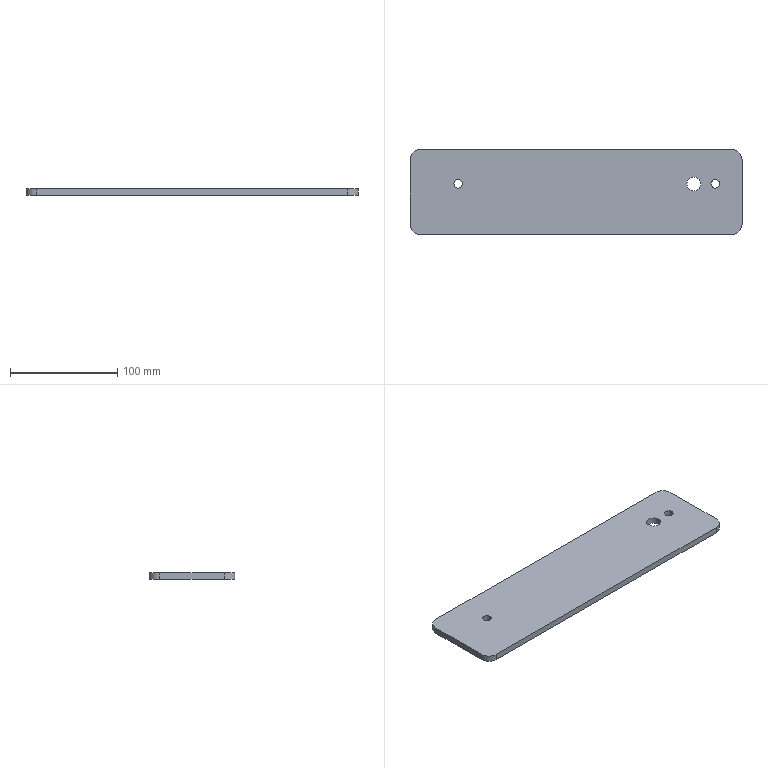Part | SolidWorks | features FlatPattern 1, SMBaseFlange 1, SheetMetal 1 | 1 solid | 16 faces | box 310 x 80 x 6 mm | volume 146885 mm3 | cylinder 10 | plane 6 | commonest cylinder face diameters 8 x4 20 x4 13 x2
STEP:
#1=CARTESIAN_POINT('',(-1216.5,-927.5,6.));
#2=VERTEX_POINT('',#1);
#3=CARTESIAN_POINT('',(-1203.5,-927.5,6.));
#4=VERTEX_POINT('',#3);
#5=CARTESIAN_POINT('',(-1210.,-927.5,6.));
#6=DIRECTION('',(0.,0.,1.));
#7=DIRECTION('',(1.,0.,0.));
#8=AXIS2_PLACEMENT_3D('',#5,#6,#7);
#9=CIRCLE('',#8,6.5);
#10=EDGE_CURVE('',#2,#4,#9,.T.);
#11=ORIENTED_EDGE('',*,*,#10,.T.);
#12=CARTESIAN_POINT('',(-1203.5,-927.5,0.));
#13=VERTEX_POINT('',#12);
#14=CARTESIAN_POINT('',(-1203.5,-927.5,6.));
#15=DIRECTION('',(0.,0.,-1.));
#16=VECTOR('',#15,1000.);
#17=LINE('',#14,#16);
#18=EDGE_CURVE('',#4,#13,#17,.T.);
#19=ORIENTED_EDGE('',*,*,#18,.T.);
#20=CARTESIAN_POINT('',(-1216.5,-927.5,0.));
#21=VERTEX_POINT('',#20);
#22=CARTESIAN_POINT('',(-1210.,-927.5,0.));
#23=DIRECTION('',(0.,0.,1.));
#24=DIRECTION('',(1.,0.,0.));
#25=AXIS2_PLACEMENT_3D('',#22,#23,#24);
#26=CIRCLE('',#25,6.5);
#27=EDGE_CURVE('',#21,#13,#26,.T.);
#28=ORIENTED_EDGE('',*,*,#27,.F.);
#29=CARTESIAN_POINT('',(-1216.5,-927.5,6.));
#30=DIRECTION('',(0.,0.,-1.));
#31=VECTOR('',#30,1000.);
#32=LINE('',#29,#31);
#33=EDGE_CURVE('',#2,#21,#32,.T.);
#34=ORIENTED_EDGE('',*,*,#33,.F.);
#35=EDGE_LOOP('',(#11,#19,#28,#34));
#36=FACE_OUTER_BOUND('',#35,.T.);
#37=CARTESIAN_POINT('',(-1210.,-927.5,6.));
#38=DIRECTION('',(0.,0.,-1.));
#39=DIRECTION('',(-1.,0.,0.));
#40=AXIS2_PLACEMENT_3D('',#37,#38,#39);
#41=CYLINDRICAL_SURFACE('',#40,6.5);
#42=ADVANCED_FACE('',(#36),#41,.F.);
#43=CARTESIAN_POINT('',(-1194.,-927.5,6.));
#44=VERTEX_POINT('',#43);
#45=CARTESIAN_POINT('',(-1186.,-927.5,6.));
#46=VERTEX_POINT('',#45);
#47=CARTESIAN_POINT('',(-1190.,-927.5,6.));
#48=DIRECTION('',(0.,0.,1.));
#49=DIRECTION('',(1.,0.,0.));
#50=AXIS2_PLACEMENT_3D('',#47,#48,#49);
#51=CIRCLE('',#50,4.);
#52=EDGE_CURVE('',#44,#46,#51,.T.);
#53=ORIENTED_EDGE('',*,*,#52,.T.);
#54=CARTESIAN_POINT('',(-1186.,-927.5,0.));
#55=VERTEX_POINT('',#54);
#56=CARTESIAN_POINT('',(-1186.,-927.5,6.));
#57=DIRECTION('',(0.,0.,-1.));
#58=VECTOR('',#57,1000.);
#59=LINE('',#56,#58);
#60=EDGE_CURVE('',#46,#55,#59,.T.);
#61=ORIENTED_EDGE('',*,*,#60,.T.);
#62=CARTESIAN_POINT('',(-1194.,-927.5,0.));
#63=VERTEX_POINT('',#62);
#64=CARTESIAN_POINT('',(-1190.,-927.5,0.));
#65=DIRECTION('',(0.,0.,1.));
#66=DIRECTION('',(1.,0.,0.));
#67=AXIS2_PLACEMENT_3D('',#64,#65,#66);
#68=CIRCLE('',#67,4.);
#69=EDGE_CURVE('',#63,#55,#68,.T.);
#70=ORIENTED_EDGE('',*,*,#69,.F.);
#71=CARTESIAN_POINT('',(-1194.,-927.5,6.));
#72=DIRECTION('',(0.,0.,-1.));
#73=VECTOR('',#72,1000.);
#74=LINE('',#71,#73);
#75=EDGE_CURVE('',#44,#63,#74,.T.);
#76=ORIENTED_EDGE('',*,*,#75,.F.);
#77=EDGE_LOOP('',(#53,#61,#70,#76));
#78=FACE_OUTER_BOUND('',#77,.T.);
#79=CARTESIAN_POINT('',(-1190.,-927.5,6.));
#80=DIRECTION('',(0.,0.,-1.));
#81=DIRECTION('',(-1.,0.,0.));
#82=AXIS2_PLACEMENT_3D('',#79,#80,#81);
#83=CYLINDRICAL_SURFACE('',#82,4.);
#84=ADVANCED_FACE('',(#78),#83,.F.);
#85=CARTESIAN_POINT('',(-1434.,-927.5,6.));
#86=VERTEX_POINT('',#85);
#87=CARTESIAN_POINT('',(-1426.,-927.5,6.));
#88=VERTEX_POINT('',#87);
#89=CARTESIAN_POINT('',(-1430.,-927.5,6.));
#90=DIRECTION('',(0.,0.,1.));
#91=DIRECTION('',(1.,0.,0.));
#92=AXIS2_PLACEMENT_3D('',#89,#90,#91);
#93=CIRCLE('',#92,4.);
#94=EDGE_CURVE('',#86,#88,#93,.T.);
#95=ORIENTED_EDGE('',*,*,#94,.T.);
#96=CARTESIAN_POINT('',(-1426.,-927.5,0.));
#97=VERTEX_POINT('',#96);
#98=CARTESIAN_POINT('',(-1426.,-927.5,6.));
#99=DIRECTION('',(0.,0.,-1.));
#100=VECTOR('',#99,1000.);
#101=LINE('',#98,#100);
#102=EDGE_CURVE('',#88,#97,#101,.T.);
#103=ORIENTED_EDGE('',*,*,#102,.T.);
#104=CARTESIAN_POINT('',(-1434.,-927.5,0.));
#105=VERTEX_POINT('',#104);
#106=CARTESIAN_POINT('',(-1430.,-927.5,0.));
#107=DIRECTION('',(0.,0.,1.));
#108=DIRECTION('',(1.,0.,0.));
#109=AXIS2_PLACEMENT_3D('',#106,#107,#108);
#110=CIRCLE('',#109,4.);
#111=EDGE_CURVE('',#105,#97,#110,.T.);
#112=ORIENTED_EDGE('',*,*,#111,.F.);
#113=CARTESIAN_POINT('',(-1434.,-927.5,6.));
#114=DIRECTION('',(0.,0.,-1.));
#115=VECTOR('',#114,1000.);
#116=LINE('',#113,#115);
#117=EDGE_CURVE('',#86,#105,#116,.T.);
#118=ORIENTED_EDGE('',*,*,#117,.F.);
#119=EDGE_LOOP('',(#95,#103,#112,#118));
#120=FACE_OUTER_BOUND('',#119,.T.);
#121=CARTESIAN_POINT('',(-1430.,-927.5,6.));
#122=DIRECTION('',(0.,0.,-1.));
#123=DIRECTION('',(-1.,0.,0.));
#124=AXIS2_PLACEMENT_3D('',#121,#122,#123);
#125=CYLINDRICAL_SURFACE('',#124,4.);
#126=ADVANCED_FACE('',(#120),#125,.F.);
#127=CARTESIAN_POINT('',(-1165.,-905.,6.));
#128=VERTEX_POINT('',#127);
#129=CARTESIAN_POINT('',(-1175.,-895.,6.));
#130=VERTEX_POINT('',#129);
#131=CARTESIAN_POINT('',(-1175.,-905.,6.));
#132=DIRECTION('',(0.,0.,1.));
#133=DIRECTION('',(-1.,0.,0.));
#134=AXIS2_PLACEMENT_3D('',#131,#132,#133);
#135=CIRCLE('',#134,10.);
#136=EDGE_CURVE('',#128,#130,#135,.T.);
#137=ORIENTED_EDGE('',*,*,#136,.T.);
#138=CARTESIAN_POINT('',(-1465.,-895.,6.));
#139=VERTEX_POINT('',#138);
#140=CARTESIAN_POINT('',(-1465.,-895.,6.));
#141=DIRECTION('',(-1.,0.,0.));
#142=VECTOR('',#141,1000.);
#143=LINE('',#140,#142);
#144=EDGE_CURVE('',#130,#139,#143,.T.);
#145=ORIENTED_EDGE('',*,*,#144,.T.);
#146=CARTESIAN_POINT('',(-1475.,-905.,6.));
#147=VERTEX_POINT('',#146);
#148=CARTESIAN_POINT('',(-1465.,-905.,6.));
#149=DIRECTION('',(0.,0.,1.));
#150=DIRECTION('',(-1.,0.,0.));
#151=AXIS2_PLACEMENT_3D('',#148,#149,#150);
#152=CIRCLE('',#151,10.);
#153=EDGE_CURVE('',#139,#147,#152,.T.);
#154=ORIENTED_EDGE('',*,*,#153,.T.);
#155=CARTESIAN_POINT('',(-1475.,-965.,6.));
#156=VERTEX_POINT('',#155);
#157=CARTESIAN_POINT('',(-1475.,-965.,6.));
#158=DIRECTION('',(0.,-1.,0.));
#159=VECTOR('',#158,1000.);
#160=LINE('',#157,#159);
#161=EDGE_CURVE('',#147,#156,#160,.T.);
#162=ORIENTED_EDGE('',*,*,#161,.T.);
#163=CARTESIAN_POINT('',(-1465.,-975.,6.));
#164=VERTEX_POINT('',#163);
#165=CARTESIAN_POINT('',(-1465.,-965.,6.));
#166=DIRECTION('',(0.,0.,1.));
#167=DIRECTION('',(-1.,0.,0.));
#168=AXIS2_PLACEMENT_3D('',#165,#166,#167);
#169=CIRCLE('',#168,10.);
#170=EDGE_CURVE('',#156,#164,#169,.T.);
#171=ORIENTED_EDGE('',*,*,#170,.T.);
#172=CARTESIAN_POINT('',(-1175.,-975.,6.));
#173=VERTEX_POINT('',#172);
#174=CARTESIAN_POINT('',(-1465.,-975.,6.));
#175=DIRECTION('',(1.,0.,0.));
#176=VECTOR('',#175,1000.);
#177=LINE('',#174,#176);
#178=EDGE_CURVE('',#164,#173,#177,.T.);
#179=ORIENTED_EDGE('',*,*,#178,.T.);
#180=CARTESIAN_POINT('',(-1165.,-965.,6.));
#181=VERTEX_POINT('',#180);
#182=CARTESIAN_POINT('',(-1175.,-965.,6.));
#183=DIRECTION('',(0.,0.,1.));
#184=DIRECTION('',(1.,0.,0.));
#185=AXIS2_PLACEMENT_3D('',#182,#183,#184);
#186=CIRCLE('',#185,10.);
#187=EDGE_CURVE('',#173,#181,#186,.T.);
#188=ORIENTED_EDGE('',*,*,#187,.T.);
#189=CARTESIAN_POINT('',(-1165.,-965.,6.));
#190=DIRECTION('',(0.,1.,0.));
#191=VECTOR('',#190,1000.);
#192=LINE('',#189,#191);
#193=EDGE_CURVE('',#181,#128,#192,.T.);
#194=ORIENTED_EDGE('',*,*,#193,.T.);
#195=EDGE_LOOP('',(#137,#145,#154,#162,#171,#179,#188,#194));
#196=FACE_OUTER_BOUND('',#195,.T.);
#197=ORIENTED_EDGE('',*,*,#94,.F.);
#198=CARTESIAN_POINT('',(-1430.,-927.5,6.));
#199=DIRECTION('',(0.,0.,1.));
#200=DIRECTION('',(1.,0.,0.));
#201=AXIS2_PLACEMENT_3D('',#198,#199,#200);
#202=CIRCLE('',#201,4.);
#203=EDGE_CURVE('',#88,#86,#202,.T.);
#204=ORIENTED_EDGE('',*,*,#203,.F.);
#205=EDGE_LOOP('',(#197,#204));
#206=FACE_BOUND('',#205,.T.);
#207=ORIENTED_EDGE('',*,*,#52,.F.);
#208=CARTESIAN_POINT('',(-1190.,-927.5,6.));
#209=DIRECTION('',(0.,0.,1.));
#210=DIRECTION('',(1.,0.,0.));
#211=AXIS2_PLACEMENT_3D('',#208,#209,#210);
#212=CIRCLE('',#211,4.);
#213=EDGE_CURVE('',#46,#44,#212,.T.);
#214=ORIENTED_EDGE('',*,*,#213,.F.);
#215=EDGE_LOOP('',(#207,#214));
#216=FACE_BOUND('',#215,.T.);
#217=ORIENTED_EDGE('',*,*,#10,.F.);
#218=CARTESIAN_POINT('',(-1210.,-927.5,6.));
#219=DIRECTION('',(0.,0.,1.));
#220=DIRECTION('',(1.,0.,0.));
#221=AXIS2_PLACEMENT_3D('',#218,#219,#220);
#222=CIRCLE('',#221,6.5);
#223=EDGE_CURVE('',#4,#2,#222,.T.);
#224=ORIENTED_EDGE('',*,*,#223,.F.);
#225=EDGE_LOOP('',(#217,#224));
#226=FACE_BOUND('',#225,.T.);
#227=CARTESIAN_POINT('',(-1175.,-905.,6.));
#228=DIRECTION('',(0.,0.,-1.));
#229=DIRECTION('',(-1.,0.,0.));
#230=AXIS2_PLACEMENT_3D('',#227,#228,#229);
#231=PLANE('',#230);
#232=ADVANCED_FACE('',(#196,#206,#216,#226),#231,.F.);
#233=ORIENTED_EDGE('',*,*,#69,.T.);
#234=CARTESIAN_POINT('',(-1190.,-927.5,0.));
#235=DIRECTION('',(0.,0.,1.));
#236=DIRECTION('',(1.,0.,0.));
#237=AXIS2_PLACEMENT_3D('',#234,#235,#236);
#238=CIRCLE('',#237,4.);
#239=EDGE_CURVE('',#55,#63,#238,.T.);
#240=ORIENTED_EDGE('',*,*,#239,.T.);
#241=EDGE_LOOP('',(#233,#240));
#242=FACE_BOUND('',#241,.T.);
#243=CARTESIAN_POINT('',(-1165.,-905.,0.));
#244=VERTEX_POINT('',#243);
#245=CARTESIAN_POINT('',(-1175.,-895.,0.));
#246=VERTEX_POINT('',#245);
#247=CARTESIAN_POINT('',(-1175.,-905.,0.));
#248=DIRECTION('',(0.,0.,1.));
#249=DIRECTION('',(-1.,0.,0.));
#250=AXIS2_PLACEMENT_3D('',#247,#248,#249);
#251=CIRCLE('',#250,10.);
#252=EDGE_CURVE('',#244,#246,#251,.T.);
#253=ORIENTED_EDGE('',*,*,#252,.F.);
#254=CARTESIAN_POINT('',(-1165.,-965.,0.));
#255=VERTEX_POINT('',#254);
#256=CARTESIAN_POINT('',(-1165.,-965.,0.));
#257=DIRECTION('',(0.,1.,0.));
#258=VECTOR('',#257,1000.);
#259=LINE('',#256,#258);
#260=EDGE_CURVE('',#255,#244,#259,.T.);
#261=ORIENTED_EDGE('',*,*,#260,.F.);
#262=CARTESIAN_POINT('',(-1175.,-975.,0.));
#263=VERTEX_POINT('',#262);
#264=CARTESIAN_POINT('',(-1175.,-965.,0.));
#265=DIRECTION('',(0.,0.,1.));
#266=DIRECTION('',(1.,0.,0.));
#267=AXIS2_PLACEMENT_3D('',#264,#265,#266);
#268=CIRCLE('',#267,10.);
#269=EDGE_CURVE('',#263,#255,#268,.T.);
#270=ORIENTED_EDGE('',*,*,#269,.F.);
#271=CARTESIAN_POINT('',(-1465.,-975.,0.));
#272=VERTEX_POINT('',#271);
#273=CARTESIAN_POINT('',(-1465.,-975.,0.));
#274=DIRECTION('',(1.,0.,0.));
#275=VECTOR('',#274,1000.);
#276=LINE('',#273,#275);
#277=EDGE_CURVE('',#272,#263,#276,.T.);
#278=ORIENTED_EDGE('',*,*,#277,.F.);
#279=CARTESIAN_POINT('',(-1475.,-965.,0.));
#280=VERTEX_POINT('',#279);
#281=CARTESIAN_POINT('',(-1465.,-965.,0.));
#282=DIRECTION('',(0.,0.,1.));
#283=DIRECTION('',(-1.,0.,0.));
#284=AXIS2_PLACEMENT_3D('',#281,#282,#283);
#285=CIRCLE('',#284,10.);
#286=EDGE_CURVE('',#280,#272,#285,.T.);
#287=ORIENTED_EDGE('',*,*,#286,.F.);
#288=CARTESIAN_POINT('',(-1475.,-905.,0.));
#289=VERTEX_POINT('',#288);
#290=CARTESIAN_POINT('',(-1475.,-965.,0.));
#291=DIRECTION('',(0.,-1.,0.));
#292=VECTOR('',#291,1000.);
#293=LINE('',#290,#292);
#294=EDGE_CURVE('',#289,#280,#293,.T.);
#295=ORIENTED_EDGE('',*,*,#294,.F.);
#296=CARTESIAN_POINT('',(-1465.,-895.,0.));
#297=VERTEX_POINT('',#296);
#298=CARTESIAN_POINT('',(-1465.,-905.,0.));
#299=DIRECTION('',(0.,0.,1.));
#300=DIRECTION('',(-1.,0.,0.));
#301=AXIS2_PLACEMENT_3D('',#298,#299,#300);
#302=CIRCLE('',#301,10.);
#303=EDGE_CURVE('',#297,#289,#302,.T.);
#304=ORIENTED_EDGE('',*,*,#303,.F.);
#305=CARTESIAN_POINT('',(-1465.,-895.,0.));
#306=DIRECTION('',(-1.,0.,0.));
#307=VECTOR('',#306,1000.);
#308=LINE('',#305,#307);
#309=EDGE_CURVE('',#246,#297,#308,.T.);
#310=ORIENTED_EDGE('',*,*,#309,.F.);
#311=EDGE_LOOP('',(#253,#261,#270,#278,#287,#295,#304,#310));
#312=FACE_OUTER_BOUND('',#311,.T.);
#313=ORIENTED_EDGE('',*,*,#111,.T.);
#314=CARTESIAN_POINT('',(-1430.,-927.5,0.));
#315=DIRECTION('',(0.,0.,1.));
#316=DIRECTION('',(1.,0.,0.));
#317=AXIS2_PLACEMENT_3D('',#314,#315,#316);
#318=CIRCLE('',#317,4.);
#319=EDGE_CURVE('',#97,#105,#318,.T.);
#320=ORIENTED_EDGE('',*,*,#319,.T.);
#321=EDGE_LOOP('',(#313,#320));
#322=FACE_BOUND('',#321,.T.);
#323=ORIENTED_EDGE('',*,*,#27,.T.);
#324=CARTESIAN_POINT('',(-1210.,-927.5,0.));
#325=DIRECTION('',(0.,0.,1.));
#326=DIRECTION('',(1.,0.,0.));
#327=AXIS2_PLACEMENT_3D('',#324,#325,#326);
#328=CIRCLE('',#327,6.5);
#329=EDGE_CURVE('',#13,#21,#328,.T.);
#330=ORIENTED_EDGE('',*,*,#329,.T.);
#331=EDGE_LOOP('',(#323,#330));
#332=FACE_BOUND('',#331,.T.);
#333=CARTESIAN_POINT('',(-1175.,-905.,0.));
#334=DIRECTION('',(0.,0.,-1.));
#335=DIRECTION('',(-1.,0.,0.));
#336=AXIS2_PLACEMENT_3D('',#333,#334,#335);
#337=PLANE('',#336);
#338=ADVANCED_FACE('',(#242,#312,#322,#332),#337,.T.);
#339=ORIENTED_EDGE('',*,*,#252,.T.);
#340=CARTESIAN_POINT('',(-1175.,-895.,6.));
#341=DIRECTION('',(0.,0.,-1.));
#342=VECTOR('',#341,1000.);
#343=LINE('',#340,#342);
#344=EDGE_CURVE('',#130,#246,#343,.T.);
#345=ORIENTED_EDGE('',*,*,#344,.F.);
#346=ORIENTED_EDGE('',*,*,#136,.F.);
#347=CARTESIAN_POINT('',(-1165.,-905.,6.));
#348=DIRECTION('',(0.,0.,-1.));
#349=VECTOR('',#348,1000.);
#350=LINE('',#347,#349);
#351=EDGE_CURVE('',#128,#244,#350,.T.);
#352=ORIENTED_EDGE('',*,*,#351,.T.);
#353=EDGE_LOOP('',(#339,#345,#346,#352));
#354=FACE_OUTER_BOUND('',#353,.T.);
#355=CARTESIAN_POINT('',(-1175.,-905.,6.));
#356=DIRECTION('',(0.,0.,-1.));
#357=DIRECTION('',(-1.,0.,0.));
#358=AXIS2_PLACEMENT_3D('',#355,#356,#357);
#359=CYLINDRICAL_SURFACE('',#358,10.);
#360=ADVANCED_FACE('',(#354),#359,.T.);
#361=ORIENTED_EDGE('',*,*,#309,.T.);
#362=CARTESIAN_POINT('',(-1465.,-895.,6.));
#363=DIRECTION('',(0.,0.,-1.));
#364=VECTOR('',#363,1000.);
#365=LINE('',#362,#364);
#366=EDGE_CURVE('',#139,#297,#365,.T.);
#367=ORIENTED_EDGE('',*,*,#366,.F.);
#368=ORIENTED_EDGE('',*,*,#144,.F.);
#369=ORIENTED_EDGE('',*,*,#344,.T.);
#370=EDGE_LOOP('',(#361,#367,#368,#369));
#371=FACE_OUTER_BOUND('',#370,.T.);
#372=CARTESIAN_POINT('',(-1465.,-895.,6.));
#373=DIRECTION('',(0.,-1.,0.));
#374=DIRECTION('',(0.,0.,-1.));
#375=AXIS2_PLACEMENT_3D('',#372,#373,#374);
#376=PLANE('',#375);
#377=ADVANCED_FACE('',(#371),#376,.F.);
#378=ORIENTED_EDGE('',*,*,#303,.T.);
#379=CARTESIAN_POINT('',(-1475.,-905.,6.));
#380=DIRECTION('',(0.,0.,-1.));
#381=VECTOR('',#380,1000.);
#382=LINE('',#379,#381);
#383=EDGE_CURVE('',#147,#289,#382,.T.);
#384=ORIENTED_EDGE('',*,*,#383,.F.);
#385=ORIENTED_EDGE('',*,*,#153,.F.);
#386=ORIENTED_EDGE('',*,*,#366,.T.);
#387=EDGE_LOOP('',(#378,#384,#385,#386));
#388=FACE_OUTER_BOUND('',#387,.T.);
#389=CARTESIAN_POINT('',(-1465.,-905.,6.));
#390=DIRECTION('',(0.,0.,-1.));
#391=DIRECTION('',(-1.,0.,0.));
#392=AXIS2_PLACEMENT_3D('',#389,#390,#391);
#393=CYLINDRICAL_SURFACE('',#392,10.);
#394=ADVANCED_FACE('',(#388),#393,.T.);
#395=ORIENTED_EDGE('',*,*,#294,.T.);
#396=CARTESIAN_POINT('',(-1475.,-965.,6.));
#397=DIRECTION('',(0.,0.,-1.));
#398=VECTOR('',#397,1000.);
#399=LINE('',#396,#398);
#400=EDGE_CURVE('',#156,#280,#399,.T.);
#401=ORIENTED_EDGE('',*,*,#400,.F.);
#402=ORIENTED_EDGE('',*,*,#161,.F.);
#403=ORIENTED_EDGE('',*,*,#383,.T.);
#404=EDGE_LOOP('',(#395,#401,#402,#403));
#405=FACE_OUTER_BOUND('',#404,.T.);
#406=CARTESIAN_POINT('',(-1475.,-965.,6.));
#407=DIRECTION('',(1.,0.,0.));
#408=DIRECTION('',(0.,0.,-1.));
#409=AXIS2_PLACEMENT_3D('',#406,#407,#408);
#410=PLANE('',#409);
#411=ADVANCED_FACE('',(#405),#410,.F.);
#412=ORIENTED_EDGE('',*,*,#286,.T.);
#413=CARTESIAN_POINT('',(-1465.,-975.,6.));
#414=DIRECTION('',(0.,0.,-1.));
#415=VECTOR('',#414,1000.);
#416=LINE('',#413,#415);
#417=EDGE_CURVE('',#164,#272,#416,.T.);
#418=ORIENTED_EDGE('',*,*,#417,.F.);
#419=ORIENTED_EDGE('',*,*,#170,.F.);
#420=ORIENTED_EDGE('',*,*,#400,.T.);
#421=EDGE_LOOP('',(#412,#418,#419,#420));
#422=FACE_OUTER_BOUND('',#421,.T.);
#423=CARTESIAN_POINT('',(-1465.,-965.,6.));
#424=DIRECTION('',(0.,0.,-1.));
#425=DIRECTION('',(-1.,0.,0.));
#426=AXIS2_PLACEMENT_3D('',#423,#424,#425);
#427=CYLINDRICAL_SURFACE('',#426,10.);
#428=ADVANCED_FACE('',(#422),#427,.T.);
#429=ORIENTED_EDGE('',*,*,#277,.T.);
#430=CARTESIAN_POINT('',(-1175.,-975.,6.));
#431=DIRECTION('',(0.,0.,-1.));
#432=VECTOR('',#431,1000.);
#433=LINE('',#430,#432);
#434=EDGE_CURVE('',#173,#263,#433,.T.);
#435=ORIENTED_EDGE('',*,*,#434,.F.);
#436=ORIENTED_EDGE('',*,*,#178,.F.);
#437=ORIENTED_EDGE('',*,*,#417,.T.);
#438=EDGE_LOOP('',(#429,#435,#436,#437));
#439=FACE_OUTER_BOUND('',#438,.T.);
#440=CARTESIAN_POINT('',(-1465.,-975.,6.));
#441=DIRECTION('',(0.,1.,0.));
#442=DIRECTION('',(0.,0.,1.));
#443=AXIS2_PLACEMENT_3D('',#440,#441,#442);
#444=PLANE('',#443);
#445=ADVANCED_FACE('',(#439),#444,.F.);
#446=ORIENTED_EDGE('',*,*,#269,.T.);
#447=CARTESIAN_POINT('',(-1165.,-965.,6.));
#448=DIRECTION('',(0.,0.,-1.));
#449=VECTOR('',#448,1000.);
#450=LINE('',#447,#449);
#451=EDGE_CURVE('',#181,#255,#450,.T.);
#452=ORIENTED_EDGE('',*,*,#451,.F.);
#453=ORIENTED_EDGE('',*,*,#187,.F.);
#454=ORIENTED_EDGE('',*,*,#434,.T.);
#455=EDGE_LOOP('',(#446,#452,#453,#454));
#456=FACE_OUTER_BOUND('',#455,.T.);
#457=CARTESIAN_POINT('',(-1175.,-965.,6.));
#458=DIRECTION('',(0.,0.,-1.));
#459=DIRECTION('',(-1.,0.,0.));
#460=AXIS2_PLACEMENT_3D('',#457,#458,#459);
#461=CYLINDRICAL_SURFACE('',#460,10.);
#462=ADVANCED_FACE('',(#456),#461,.T.);
#463=ORIENTED_EDGE('',*,*,#260,.T.);
#464=ORIENTED_EDGE('',*,*,#351,.F.);
#465=ORIENTED_EDGE('',*,*,#193,.F.);
#466=ORIENTED_EDGE('',*,*,#451,.T.);
#467=EDGE_LOOP('',(#463,#464,#465,#466));
#468=FACE_OUTER_BOUND('',#467,.T.);
#469=CARTESIAN_POINT('',(-1165.,-965.,6.));
#470=DIRECTION('',(-1.,0.,0.));
#471=DIRECTION('',(0.,0.,1.));
#472=AXIS2_PLACEMENT_3D('',#469,#470,#471);
#473=PLANE('',#472);
#474=ADVANCED_FACE('',(#468),#473,.F.);
#475=ORIENTED_EDGE('',*,*,#102,.F.);
#476=ORIENTED_EDGE('',*,*,#203,.T.);
#477=ORIENTED_EDGE('',*,*,#117,.T.);
#478=ORIENTED_EDGE('',*,*,#319,.F.);
#479=EDGE_LOOP('',(#475,#476,#477,#478));
#480=FACE_OUTER_BOUND('',#479,.T.);
#481=CARTESIAN_POINT('',(-1430.,-927.5,6.));
#482=DIRECTION('',(0.,0.,-1.));
#483=DIRECTION('',(-1.,0.,0.));
#484=AXIS2_PLACEMENT_3D('',#481,#482,#483);
#485=CYLINDRICAL_SURFACE('',#484,4.);
#486=ADVANCED_FACE('',(#480),#485,.F.);
#487=ORIENTED_EDGE('',*,*,#60,.F.);
#488=ORIENTED_EDGE('',*,*,#213,.T.);
#489=ORIENTED_EDGE('',*,*,#75,.T.);
#490=ORIENTED_EDGE('',*,*,#239,.F.);
#491=EDGE_LOOP('',(#487,#488,#489,#490));
#492=FACE_OUTER_BOUND('',#491,.T.);
#493=CARTESIAN_POINT('',(-1190.,-927.5,6.));
#494=DIRECTION('',(0.,0.,-1.));
#495=DIRECTION('',(-1.,0.,0.));
#496=AXIS2_PLACEMENT_3D('',#493,#494,#495);
#497=CYLINDRICAL_SURFACE('',#496,4.);
#498=ADVANCED_FACE('',(#492),#497,.F.);
#499=ORIENTED_EDGE('',*,*,#18,.F.);
#500=ORIENTED_EDGE('',*,*,#223,.T.);
#501=ORIENTED_EDGE('',*,*,#33,.T.);
#502=ORIENTED_EDGE('',*,*,#329,.F.);
#503=EDGE_LOOP('',(#499,#500,#501,#502));
#504=FACE_OUTER_BOUND('',#503,.T.);
#505=CARTESIAN_POINT('',(-1210.,-927.5,6.));
#506=DIRECTION('',(0.,0.,-1.));
#507=DIRECTION('',(-1.,0.,0.));
#508=AXIS2_PLACEMENT_3D('',#505,#506,#507);
#509=CYLINDRICAL_SURFACE('',#508,6.5);
#510=ADVANCED_FACE('',(#504),#509,.F.);
#511=CLOSED_SHELL('',(#42,#84,#126,#232,#338,#360,#377,#394,#411,#428,#445,#462,#474,#486,#498,#510));
#512=MANIFOLD_SOLID_BREP('',#511);
#513=CARTESIAN_POINT('',(0.,0.,0.));
#514=DIRECTION('',(0.,0.,1.));
#515=DIRECTION('',(1.,0.,0.));
#516=AXIS2_PLACEMENT_3D('',#513,#514,#515);
#517=(LENGTH_UNIT()NAMED_UNIT(*)SI_UNIT(.MILLI.,.METRE.));
#518=UNCERTAINTY_MEASURE_WITH_UNIT(LENGTH_MEASURE(0.00001),#517,'','');
#519=(NAMED_UNIT(*)PLANE_ANGLE_UNIT()SI_UNIT($,.RADIAN.));
#520=(NAMED_UNIT(*)SI_UNIT($,.STERADIAN.)SOLID_ANGLE_UNIT());
#521=(GEOMETRIC_REPRESENTATION_CONTEXT(3)GLOBAL_UNCERTAINTY_ASSIGNED_CONTEXT((#518))GLOBAL_UNIT_ASSIGNED_CONTEXT((#517,#519,#520))REPRESENTATION_CONTEXT('',''));
#522=ADVANCED_BREP_SHAPE_REPRESENTATION('',(#512,#516),#521);